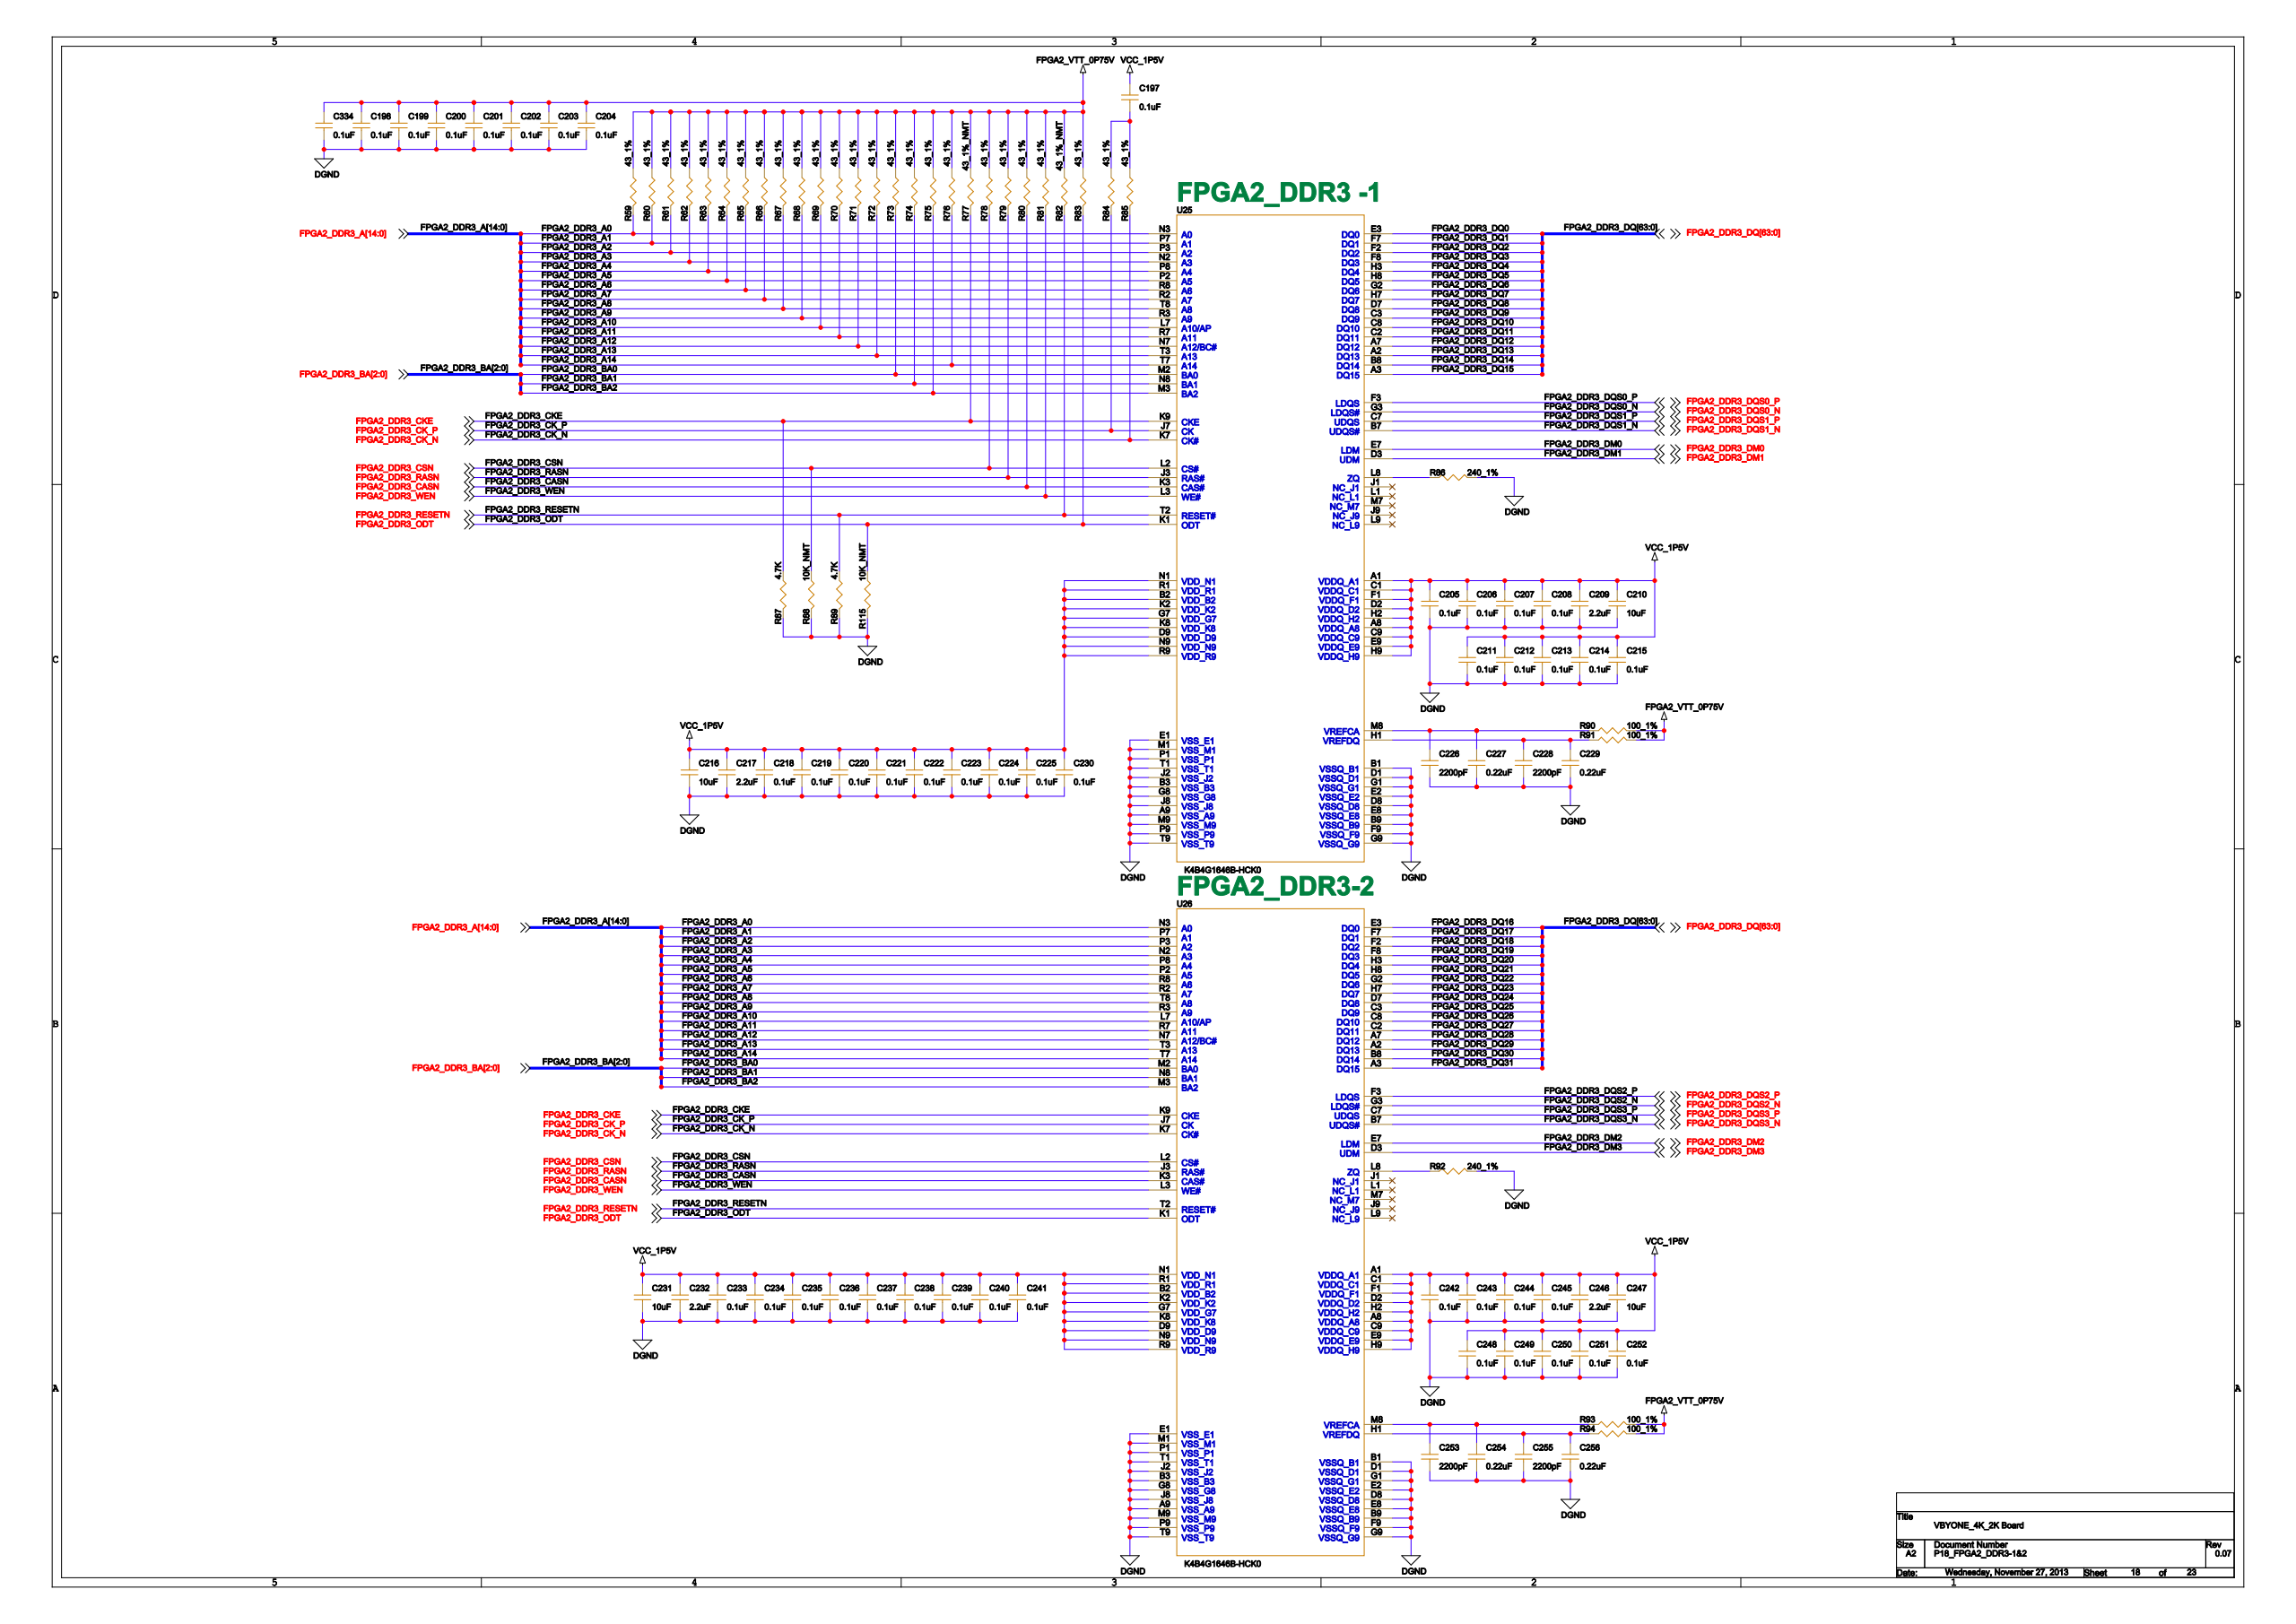Circuit board | Cadence Allegro | 1712 parts | 1495 nets | one sheet of the schematic
Parts on this sheet (reference | value | footprint):
C197 | 0.1uF | CRC1005RZAS
C198 | 0.1uF | CRC1005RZAS
C199 | 0.1uF | CRC1005RZAS
C200 | 0.1uF | CRC1005RZAS
C201 | 0.1uF | CRC1005RZAS
C202 | 0.1uF | CRC1005RZAS
C203 | 0.1uF | CRC1005RZAS
C204 | 0.1uF | CRC1005RZAS
C205 | 0.1uF | CRC1005RZAS
C206 | 0.1uF | CRC1005RZAS
C207 | 0.1uF | CRC1005RZAS
C208 | 0.1uF | CRC1005RZAS
C209 | 2.2uF | CRC1608RZAS
C210 | 10uF | CRC2012RZAS
C211 | 0.1uF | CRC1005RZAS
C212 | 0.1uF | CRC1005RZAS
C213 | 0.1uF | CRC1005RZAS
C214 | 0.1uF | CRC1005RZAS
C215 | 0.1uF | CRC1005RZAS
C216 | 10uF | CRC2012RZAS
C217 | 2.2uF | CRC1608RZAS
C218 | 0.1uF | CRC1005RZAS
C219 | 0.1uF | CRC1005RZAS
C220 | 0.1uF | CRC1005RZAS
C221 | 0.1uF | CRC1005RZAS
C222 | 0.1uF | CRC1005RZAS
C223 | 0.1uF | CRC1005RZAS
C224 | 0.1uF | CRC1005RZAS
C225 | 0.1uF | CRC1005RZAS
C226 | 2200pF | CRC1608RZAS
C227 | 0.22uF | CRC1608RZAS
C228 | 2200pF | CRC1608RZAS
C229 | 0.22uF | CRC1608RZAS
C230 | 0.1uF | CRC1005RZAS
C231 | 10uF | CRC2012RZAS
C232 | 2.2uF | CRC1608RZAS
C233 | 0.1uF | CRC1005RZAS
C234 | 0.1uF | CRC1005RZAS
C235 | 0.1uF | CRC1005RZAS
C236 | 0.1uF | CRC1005RZAS
C237 | 0.1uF | CRC1005RZAS
C238 | 0.1uF | CRC1005RZAS
C239 | 0.1uF | CRC1005RZAS
C240 | 0.1uF | CRC1005RZAS
C241 | 0.1uF | CRC1005RZAS
C242 | 0.1uF | CRC1005RZAS
C243 | 0.1uF | CRC1005RZAS
C244 | 0.1uF | CRC1005RZAS
C245 | 0.1uF | CRC1005RZAS
C246 | 2.2uF | CRC1608RZAS
C247 | 10uF | CRC2012RZAS
C248 | 0.1uF | CRC1005RZAS
C249 | 0.1uF | CRC1005RZAS
C250 | 0.1uF | CRC1005RZAS
C251 | 0.1uF | CRC1005RZAS
C252 | 0.1uF | CRC1005RZAS
C253 | 2200pF | CRC1608RZAS
C254 | 0.22uF | CRC1608RZAS
C255 | 2200pF | CRC1608RZAS
C256 | 0.22uF | CRC1608RZAS
C334 | 0.1uF | CRC1005RZAS
R59 | 43_1% | CRC1005RZAS
R60 | 43_1% | CRC1005RZAS
R61 | 43_1% | CRC1005RZAS
R62 | 43_1% | CRC1005RZAS
R63 | 43_1% | CRC1005RZAS
R64 | 43_1% | CRC1005RZAS
R65 | 43_1% | CRC1005RZAS
R66 | 43_1% | CRC1005RZAS
R67 | 43_1% | CRC1005RZAS
R68 | 43_1% | CRC1005RZAS
R69 | 43_1% | CRC1005RZAS
R70 | 43_1% | CRC1005RZAS
R71 | 43_1% | CRC1005RZAS
R72 | 43_1% | CRC1005RZAS
R73 | 43_1% | CRC1005RZAS
R74 | 43_1% | CRC1005RZAS
R75 | 43_1% | CRC1005RZAS
R76 | 43_1% | CRC1005RZAS
R77 | 43_1%_NMT | CRC1005RZAS
R78 | 43_1% | CRC1005RZAS
R79 | 43_1% | CRC1005RZAS
R80 | 43_1% | CRC1005RZAS
R81 | 43_1% | CRC1005RZAS
R82 | 43_1%_NMT | CRC1005RZAS
R83 | 43_1% | CRC1005RZAS
R84 | 43_1% | CRC1005RZAS
R85 | 43_1% | CRC1005RZAS
R86 | 240_1% | CRC1608RZAS
R87 | 4.7K | CRC1005RZAS
R88 | 10K_NMT | CRC1005RZAS
R89 | 4.7K | CRC1005RZAS
R90 | 100_1% | CRC1005RZAS
R91 | 100_1% | CRC1005RZAS
R92 | 240_1% | CRC1608RZAS
R93 | 100_1% | CRC1005RZAS
R94 | 100_1% | CRC1005RZAS
R115 | 10K_NMT | CRC1005RZAS
U25 | K4B4G1646B-HCK0 | BGA096RFDS
U26 | K4B4G1646B-HCK0 | BGA096RFDS
Nets of these parts (net: part-pin ...):
DGND: C198-2 C199-2 C200-2 C201-2 C202-2 C203-2 C204-2 C205-2 C206-2 C207-2 C208-2 C209-2 C210-2 C211-2 C212-2 C213-2 C214-2 C215-2 C216-2 C217-2 C218-2 C219-2 C220-2 C221-2 C222-2 C223-2 C224-2 C225-2 C226-2 C227-2 C228-2 C229-2 C230-2 C231-2 C232-2 C233-2 C234-2 C235-2 C236-2 C237-2 C238-2 C239-2 C240-2 C241-2 C242-2 C243-2 C244-2 C245-2 C246-2 C247-2 C248-2 C249-2 C250-2 C251-2 C252-2 C253-2 C254-2 C255-2 C256-2 C334-2 R86-2 R87-2 R88-2 R89-2 R92-2 R115-2 U25-A9 U25-B1 U25-B3 U25-B9 U25-D1 U25-D8 U25-E1 U25-E2 U25-E8 U25-F9 U25-G1 U25-G8 U25-G9 U25-J2 U25-J8 U25-M1 U25-M9 U25-P1 U25-P9 U25-T1 U25-T9 U26-A9 U26-B1 U26-B3 U26-B9 U26-D1 U26-D8 U26-E1 U26-E2 U26-E8 U26-F9 U26-G1 U26-G8 U26-G9 U26-J2 U26-J8 U26-M1 U26-M9 U26-P1 U26-P9 U26-T1 U26-T9
VCC_1P5V: C197-1 C205-1 C206-1 C207-1 C208-1 C209-1 C210-1 C211-1 C212-1 C213-1 C214-1 C215-1 C216-1 C217-1 C218-1 C219-1 C220-1 C221-1 C222-1 C223-1 C224-1 C225-1 C230-1 C231-1 C232-1 C233-1 C234-1 C235-1 C236-1 C237-1 C238-1 C239-1 C240-1 C241-1 C242-1 C243-1 C244-1 C245-1 C246-1 C247-1 C248-1 C249-1 C250-1 C251-1 C252-1 U25-A1 U25-A8 U25-B2 U25-C1 U25-C9 U25-D2 U25-D9 U25-E9 U25-F1 U25-G7 U25-H2 U25-H9 U25-K2 U25-K8 U25-N1 U25-N9 U25-R1 U25-R9 U26-A1 U26-A8 U26-B2 U26-C1 U26-C9 U26-D2 U26-D9 U26-E9 U26-F1 U26-G7 U26-H2 U26-H9 U26-K2 U26-K8 U26-N1 U26-N9 U26-R1 U26-R9
FPGA2_VTT_0P75V: C198-1 C199-1 C200-1 C201-1 C202-1 C203-1 C204-1 C334-1 R59-1 R60-1 R61-1 R62-1 R63-1 R64-1 R65-1 R66-1 R67-1 R68-1 R69-1 R70-1 R71-1 R72-1 R73-1 R74-1 R75-1 R76-1 R77-1 R78-1 R79-1 R80-1 R81-1 R82-1 R83-1 R90-2 R91-2 R93-2 R94-2
N15827286: C197-2 R84-1 R85-1
N15826022: C226-1 C227-1 R90-1 U25-M8
N15826046: C228-1 C229-1 R91-1 U25-H1
N15827802: C253-1 C254-1 R93-1 U26-M8
N15828084: C255-1 C256-1 R94-1 U26-H1
FPGA2_DDR3_CKE: R77-2 R87-1 U25-K9 U26-K9
FPGA2_DDR3_RESETN: R82-2 R89-1 U25-T2 U26-T2
FPGA2_DDR3_ODT: R83-2 R115-1 U25-K1 U26-K1
FPGA2_DDR3_CSN: R78-2 R88-1 U25-L2 U26-L2
FPGA2_DDR3_A0: R59-2 U25-N3 U26-N3
FPGA2_DDR3_A1: R60-2 U25-P7 U26-P7
FPGA2_DDR3_A2: R61-2 U25-P3 U26-P3
FPGA2_DDR3_A3: R62-2 U25-N2 U26-N2
FPGA2_DDR3_A4: R63-2 U25-P8 U26-P8
FPGA2_DDR3_A5: R64-2 U25-P2 U26-P2
FPGA2_DDR3_A6: R65-2 U25-R8 U26-R8
FPGA2_DDR3_A7: R66-2 U25-R2 U26-R2
FPGA2_DDR3_A8: R67-2 U25-T8 U26-T8
FPGA2_DDR3_A9: R68-2 U25-R3 U26-R3
FPGA2_DDR3_A10: R69-2 U25-L7 U26-L7
FPGA2_DDR3_A11: R70-2 U25-R7 U26-R7
FPGA2_DDR3_A12: R71-2 U25-N7 U26-N7
FPGA2_DDR3_A13: R72-2 U25-T3 U26-T3
FPGA2_DDR3_BA0: R73-2 U25-M2 U26-M2
FPGA2_DDR3_BA1: R74-2 U25-N8 U26-N8
FPGA2_DDR3_BA2: R75-2 U25-M3 U26-M3
FPGA2_DDR3_A14: R76-2 U25-T7 U26-T7
FPGA2_DDR3_RASN: R79-2 U25-J3 U26-J3
FPGA2_DDR3_CASN: R80-2 U25-K3 U26-K3
FPGA2_DDR3_WEN: R81-2 U25-L3 U26-L3
FPGA2_DDR3_CK_P: R84-2 U25-J7 U26-J7
FPGA2_DDR3_CK_N: R85-2 U25-K7 U26-K7
N15830038: R86-1 U25-L8
N15830686: R92-1 U26-L8
FPGA2_DDR3_DQ22: U26-G2
FPGA2_DDR3_DQ21: U26-H8
FPGA2_DDR3_DQS2_N: U26-G3
FPGA2_DDR3_DQ10: U25-C8
FPGA2_DDR3_DQ9: U25-C3
FPGA2_DDR3_DQS0_N: U25-G3
FPGA2_DDR3_DQ2: U25-F2
FPGA2_DDR3_DQ20: U26-H3
FPGA2_DDR3_DQ19: U26-F8
FPGA2_DDR3_DQS2_P: U26-F3
FPGA2_DDR3_DQ8: U25-D7
FPGA2_DDR3_DQS0_P: U25-F3
FPGA2_DDR3_DQ1: U25-F7
FPGA2_DDR3_DQ23: U26-H7
FPGA2_DDR3_DQS1_N: U25-B7
FPGA2_DDR3_DM1: U25-D3
FPGA2_DDR3_DQ12: U25-A7
FPGA2_DDR3_DQ0: U25-E3
FPGA2_DDR3_DQ31: U26-A3
FPGA2_DDR3_DQ16: U26-E3
FPGA2_DDR3_DM2: U26-E7
FPGA2_DDR3_DQS1_P: U25-C7
FPGA2_DDR3_DQ11: U25-C2
FPGA2_DDR3_DM0: U25-E7
FPGA2_DDR3_DQ4: U25-H3
FPGA2_DDR3_DQ30: U26-B8
FPGA2_DDR3_DQ18: U26-F2
FPGA2_DDR3_DQ14: U25-B8
FPGA2_DDR3_DQ13: U25-A2
FPGA2_DDR3_DQ3: U25-F8
FPGA2_DDR3_DQ27: U26-C2
FPGA2_DDR3_DQ26: U26-C8
FPGA2_DDR3_DQ17: U26-F7
FPGA2_DDR3_DQ15: U25-A3
FPGA2_DDR3_DQ6: U25-G2
FPGA2_DDR3_DQ5: U25-H8
FPGA2_DDR3_DQS3_N: U26-B7
FPGA2_DDR3_DQS3_P: U26-C7
FPGA2_DDR3_DQ25: U26-C3
FPGA2_DDR3_DQ24: U26-D7
FPGA2_DDR3_DQ7: U25-H7
FPGA2_DDR3_DQ29: U26-A2
FPGA2_DDR3_DQ28: U26-A7
FPGA2_DDR3_DM3: U26-D3